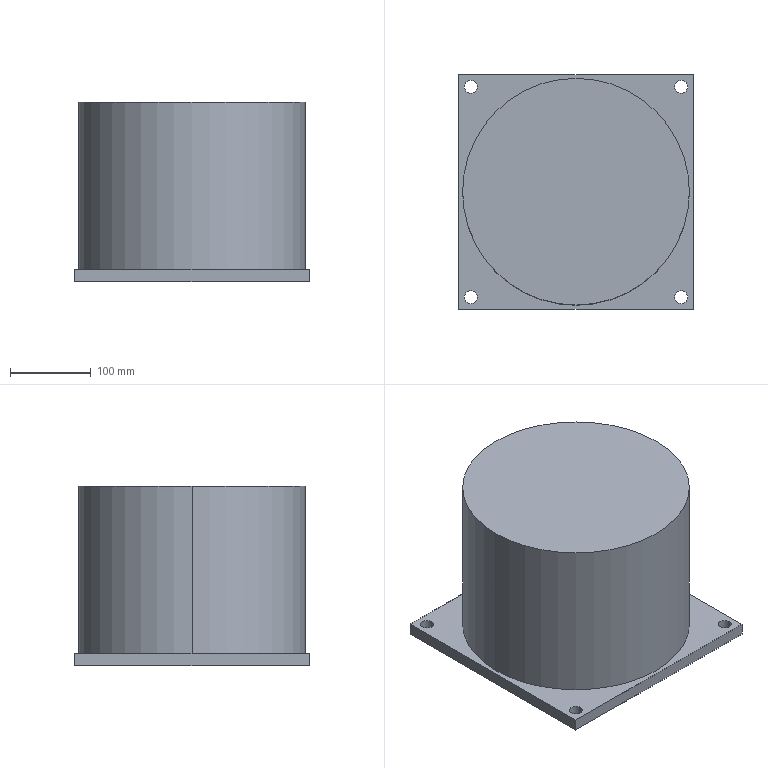Part | NX | 1 solid | 17 faces | box 290 x 290 x 222 mm | volume 13995506 mm3 | cylinder 10 | plane 7 | commonest cylinder face diameters 16 x8 280 x2
STEP:
#1=CARTESIAN_POINT('',(-35.226,-137.015,29.));
#2=VERTEX_POINT('',#1);
#3=CARTESIAN_POINT('',(-315.226,-137.015,29.));
#4=VERTEX_POINT('',#3);
#5=CARTESIAN_POINT('',(-175.226,-137.015,29.));
#6=DIRECTION('',(0.,0.,-1.));
#7=DIRECTION('',(-1.,0.,0.));
#8=AXIS2_PLACEMENT_3D('',#5,#6,#7);
#9=CIRCLE('',#8,140.);
#10=EDGE_CURVE('',#2,#4,#9,.T.);
#11=ORIENTED_EDGE('',*,*,#10,.F.);
#12=CARTESIAN_POINT('',(-35.226,-137.015,236.));
#13=VERTEX_POINT('',#12);
#14=CARTESIAN_POINT('',(-35.226,-137.015,236.));
#15=DIRECTION('',(0.,0.,-1.));
#16=VECTOR('',#15,1000.);
#17=LINE('',#14,#16);
#18=EDGE_CURVE('',#2,#13,#17,.F.);
#19=ORIENTED_EDGE('',*,*,#18,.T.);
#20=CARTESIAN_POINT('',(-315.226,-137.015,236.));
#21=VERTEX_POINT('',#20);
#22=CARTESIAN_POINT('',(-175.226,-137.015,236.));
#23=DIRECTION('',(0.,0.,-1.));
#24=DIRECTION('',(-1.,0.,0.));
#25=AXIS2_PLACEMENT_3D('',#22,#23,#24);
#26=CIRCLE('',#25,140.);
#27=EDGE_CURVE('',#13,#21,#26,.T.);
#28=ORIENTED_EDGE('',*,*,#27,.T.);
#29=CARTESIAN_POINT('',(-315.226,-137.015,236.));
#30=DIRECTION('',(0.,0.,-1.));
#31=VECTOR('',#30,1000.);
#32=LINE('',#29,#31);
#33=EDGE_CURVE('',#4,#21,#32,.F.);
#34=ORIENTED_EDGE('',*,*,#33,.F.);
#35=EDGE_LOOP('',(#11,#19,#28,#34));
#36=FACE_BOUND('',#35,.T.);
#37=CARTESIAN_POINT('',(-175.226,-137.015,236.));
#38=DIRECTION('',(0.,0.,-1.));
#39=DIRECTION('',(-1.,0.,0.));
#40=AXIS2_PLACEMENT_3D('',#37,#38,#39);
#41=CYLINDRICAL_SURFACE('',#40,140.);
#42=ADVANCED_FACE('',(#36),#41,.T.);
#43=CARTESIAN_POINT('',(-320.226,-282.015,29.));
#44=VERTEX_POINT('',#43);
#45=CARTESIAN_POINT('',(-320.226,7.985,29.));
#46=VERTEX_POINT('',#45);
#47=CARTESIAN_POINT('',(-320.226,-137.015,29.));
#48=DIRECTION('',(0.,1.,0.));
#49=VECTOR('',#48,1000.);
#50=LINE('',#47,#49);
#51=EDGE_CURVE('',#44,#46,#50,.T.);
#52=ORIENTED_EDGE('',*,*,#51,.F.);
#53=CARTESIAN_POINT('',(-30.226,-282.015,29.));
#54=VERTEX_POINT('',#53);
#55=CARTESIAN_POINT('',(-175.226,-282.015,29.));
#56=DIRECTION('',(-1.,0.,0.));
#57=VECTOR('',#56,1000.);
#58=LINE('',#55,#57);
#59=EDGE_CURVE('',#54,#44,#58,.T.);
#60=ORIENTED_EDGE('',*,*,#59,.F.);
#61=CARTESIAN_POINT('',(-30.226,7.985,29.));
#62=VERTEX_POINT('',#61);
#63=CARTESIAN_POINT('',(-30.226,-137.015,29.));
#64=DIRECTION('',(0.,1.,0.));
#65=VECTOR('',#64,1000.);
#66=LINE('',#63,#65);
#67=EDGE_CURVE('',#54,#62,#66,.T.);
#68=ORIENTED_EDGE('',*,*,#67,.T.);
#69=CARTESIAN_POINT('',(-175.226,7.985,29.));
#70=DIRECTION('',(-1.,0.,0.));
#71=VECTOR('',#70,1000.);
#72=LINE('',#69,#71);
#73=EDGE_CURVE('',#62,#46,#72,.T.);
#74=ORIENTED_EDGE('',*,*,#73,.T.);
#75=EDGE_LOOP('',(#52,#60,#68,#74));
#76=FACE_BOUND('',#75,.T.);
#77=CARTESIAN_POINT('',(-37.226,-267.015,29.));
#78=VERTEX_POINT('',#77);
#79=CARTESIAN_POINT('',(-53.226,-267.015,29.));
#80=VERTEX_POINT('',#79);
#81=CARTESIAN_POINT('',(-45.226,-267.015,29.));
#82=DIRECTION('',(0.,0.,-1.));
#83=DIRECTION('',(-1.,0.,0.));
#84=AXIS2_PLACEMENT_3D('',#81,#82,#83);
#85=CIRCLE('',#84,8.);
#86=EDGE_CURVE('',#78,#80,#85,.T.);
#87=ORIENTED_EDGE('',*,*,#86,.T.);
#88=CARTESIAN_POINT('',(-45.226,-267.015,29.));
#89=DIRECTION('',(0.,0.,-1.));
#90=DIRECTION('',(-1.,0.,0.));
#91=AXIS2_PLACEMENT_3D('',#88,#89,#90);
#92=CIRCLE('',#91,8.);
#93=EDGE_CURVE('',#80,#78,#92,.T.);
#94=ORIENTED_EDGE('',*,*,#93,.T.);
#95=EDGE_LOOP('',(#87,#94));
#96=FACE_BOUND('',#95,.T.);
#97=CARTESIAN_POINT('',(-297.226,-267.015,29.));
#98=VERTEX_POINT('',#97);
#99=CARTESIAN_POINT('',(-313.226,-267.015,29.));
#100=VERTEX_POINT('',#99);
#101=CARTESIAN_POINT('',(-305.226,-267.015,29.));
#102=DIRECTION('',(0.,0.,-1.));
#103=DIRECTION('',(-1.,0.,0.));
#104=AXIS2_PLACEMENT_3D('',#101,#102,#103);
#105=CIRCLE('',#104,8.);
#106=EDGE_CURVE('',#98,#100,#105,.T.);
#107=ORIENTED_EDGE('',*,*,#106,.T.);
#108=CARTESIAN_POINT('',(-305.226,-267.015,29.));
#109=DIRECTION('',(0.,0.,-1.));
#110=DIRECTION('',(-1.,0.,0.));
#111=AXIS2_PLACEMENT_3D('',#108,#109,#110);
#112=CIRCLE('',#111,8.);
#113=EDGE_CURVE('',#100,#98,#112,.T.);
#114=ORIENTED_EDGE('',*,*,#113,.T.);
#115=EDGE_LOOP('',(#107,#114));
#116=FACE_BOUND('',#115,.T.);
#117=CARTESIAN_POINT('',(-37.226,-7.015,29.));
#118=VERTEX_POINT('',#117);
#119=CARTESIAN_POINT('',(-53.226,-7.015,29.));
#120=VERTEX_POINT('',#119);
#121=CARTESIAN_POINT('',(-45.226,-7.015,29.));
#122=DIRECTION('',(0.,0.,-1.));
#123=DIRECTION('',(-1.,0.,0.));
#124=AXIS2_PLACEMENT_3D('',#121,#122,#123);
#125=CIRCLE('',#124,8.);
#126=EDGE_CURVE('',#118,#120,#125,.T.);
#127=ORIENTED_EDGE('',*,*,#126,.T.);
#128=CARTESIAN_POINT('',(-45.226,-7.015,29.));
#129=DIRECTION('',(0.,0.,-1.));
#130=DIRECTION('',(-1.,0.,0.));
#131=AXIS2_PLACEMENT_3D('',#128,#129,#130);
#132=CIRCLE('',#131,8.);
#133=EDGE_CURVE('',#120,#118,#132,.T.);
#134=ORIENTED_EDGE('',*,*,#133,.T.);
#135=EDGE_LOOP('',(#127,#134));
#136=FACE_BOUND('',#135,.T.);
#137=CARTESIAN_POINT('',(-297.226,-7.015,29.));
#138=VERTEX_POINT('',#137);
#139=CARTESIAN_POINT('',(-313.226,-7.015,29.));
#140=VERTEX_POINT('',#139);
#141=CARTESIAN_POINT('',(-305.226,-7.015,29.));
#142=DIRECTION('',(0.,0.,-1.));
#143=DIRECTION('',(-1.,0.,0.));
#144=AXIS2_PLACEMENT_3D('',#141,#142,#143);
#145=CIRCLE('',#144,8.);
#146=EDGE_CURVE('',#138,#140,#145,.T.);
#147=ORIENTED_EDGE('',*,*,#146,.T.);
#148=CARTESIAN_POINT('',(-305.226,-7.015,29.));
#149=DIRECTION('',(0.,0.,-1.));
#150=DIRECTION('',(-1.,0.,0.));
#151=AXIS2_PLACEMENT_3D('',#148,#149,#150);
#152=CIRCLE('',#151,8.);
#153=EDGE_CURVE('',#140,#138,#152,.T.);
#154=ORIENTED_EDGE('',*,*,#153,.T.);
#155=EDGE_LOOP('',(#147,#154));
#156=FACE_BOUND('',#155,.T.);
#157=ORIENTED_EDGE('',*,*,#10,.T.);
#158=CARTESIAN_POINT('',(-175.226,-137.015,29.));
#159=DIRECTION('',(0.,0.,-1.));
#160=DIRECTION('',(-1.,0.,0.));
#161=AXIS2_PLACEMENT_3D('',#158,#159,#160);
#162=CIRCLE('',#161,140.);
#163=EDGE_CURVE('',#4,#2,#162,.T.);
#164=ORIENTED_EDGE('',*,*,#163,.T.);
#165=EDGE_LOOP('',(#157,#164));
#166=FACE_BOUND('',#165,.T.);
#167=CARTESIAN_POINT('',(-181.149,-97.75,29.));
#168=DIRECTION('',(0.,0.,-1.));
#169=DIRECTION('',(0.,-1.,0.));
#170=AXIS2_PLACEMENT_3D('',#167,#168,#169);
#171=PLANE('',#170);
#172=ADVANCED_FACE('',(#76,#96,#116,#136,#156,#166),#171,.F.);
#173=ORIENTED_EDGE('',*,*,#73,.F.);
#174=CARTESIAN_POINT('',(-30.226,7.985,14.));
#175=VERTEX_POINT('',#174);
#176=CARTESIAN_POINT('',(-30.226,7.985,29.));
#177=DIRECTION('',(0.,0.,-1.));
#178=VECTOR('',#177,1000.);
#179=LINE('',#176,#178);
#180=EDGE_CURVE('',#62,#175,#179,.T.);
#181=ORIENTED_EDGE('',*,*,#180,.T.);
#182=CARTESIAN_POINT('',(-320.226,7.985,14.));
#183=VERTEX_POINT('',#182);
#184=CARTESIAN_POINT('',(-175.226,7.985,14.));
#185=DIRECTION('',(-1.,0.,0.));
#186=VECTOR('',#185,1000.);
#187=LINE('',#184,#186);
#188=EDGE_CURVE('',#175,#183,#187,.T.);
#189=ORIENTED_EDGE('',*,*,#188,.T.);
#190=CARTESIAN_POINT('',(-320.226,7.985,29.));
#191=DIRECTION('',(0.,0.,-1.));
#192=VECTOR('',#191,1000.);
#193=LINE('',#190,#192);
#194=EDGE_CURVE('',#46,#183,#193,.T.);
#195=ORIENTED_EDGE('',*,*,#194,.F.);
#196=EDGE_LOOP('',(#173,#181,#189,#195));
#197=FACE_BOUND('',#196,.T.);
#198=CARTESIAN_POINT('',(-30.226,7.985,29.));
#199=DIRECTION('',(0.,1.,0.));
#200=DIRECTION('',(1.,0.,0.));
#201=AXIS2_PLACEMENT_3D('',#198,#199,#200);
#202=PLANE('',#201);
#203=ADVANCED_FACE('',(#197),#202,.T.);
#204=ORIENTED_EDGE('',*,*,#59,.T.);
#205=CARTESIAN_POINT('',(-320.226,-282.015,14.));
#206=VERTEX_POINT('',#205);
#207=CARTESIAN_POINT('',(-320.226,-282.015,29.));
#208=DIRECTION('',(0.,0.,-1.));
#209=VECTOR('',#208,1000.);
#210=LINE('',#207,#209);
#211=EDGE_CURVE('',#44,#206,#210,.T.);
#212=ORIENTED_EDGE('',*,*,#211,.T.);
#213=CARTESIAN_POINT('',(-30.226,-282.015,14.));
#214=VERTEX_POINT('',#213);
#215=CARTESIAN_POINT('',(-175.226,-282.015,14.));
#216=DIRECTION('',(-1.,0.,0.));
#217=VECTOR('',#216,1000.);
#218=LINE('',#215,#217);
#219=EDGE_CURVE('',#214,#206,#218,.T.);
#220=ORIENTED_EDGE('',*,*,#219,.F.);
#221=CARTESIAN_POINT('',(-30.226,-282.015,29.));
#222=DIRECTION('',(0.,0.,-1.));
#223=VECTOR('',#222,1000.);
#224=LINE('',#221,#223);
#225=EDGE_CURVE('',#54,#214,#224,.T.);
#226=ORIENTED_EDGE('',*,*,#225,.F.);
#227=EDGE_LOOP('',(#204,#212,#220,#226));
#228=FACE_BOUND('',#227,.T.);
#229=CARTESIAN_POINT('',(-320.226,-282.015,29.));
#230=DIRECTION('',(0.,-1.,0.));
#231=DIRECTION('',(0.,0.,-1.));
#232=AXIS2_PLACEMENT_3D('',#229,#230,#231);
#233=PLANE('',#232);
#234=ADVANCED_FACE('',(#228),#233,.T.);
#235=ORIENTED_EDGE('',*,*,#67,.F.);
#236=ORIENTED_EDGE('',*,*,#225,.T.);
#237=CARTESIAN_POINT('',(-30.226,-137.015,14.));
#238=DIRECTION('',(0.,1.,0.));
#239=VECTOR('',#238,1000.);
#240=LINE('',#237,#239);
#241=EDGE_CURVE('',#214,#175,#240,.T.);
#242=ORIENTED_EDGE('',*,*,#241,.T.);
#243=ORIENTED_EDGE('',*,*,#180,.F.);
#244=EDGE_LOOP('',(#235,#236,#242,#243));
#245=FACE_BOUND('',#244,.T.);
#246=CARTESIAN_POINT('',(-30.226,-282.015,29.));
#247=DIRECTION('',(1.,0.,0.));
#248=DIRECTION('',(0.,1.,0.));
#249=AXIS2_PLACEMENT_3D('',#246,#247,#248);
#250=PLANE('',#249);
#251=ADVANCED_FACE('',(#245),#250,.T.);
#252=ORIENTED_EDGE('',*,*,#51,.T.);
#253=ORIENTED_EDGE('',*,*,#194,.T.);
#254=CARTESIAN_POINT('',(-320.226,-137.015,14.));
#255=DIRECTION('',(0.,1.,0.));
#256=VECTOR('',#255,1000.);
#257=LINE('',#254,#256);
#258=EDGE_CURVE('',#206,#183,#257,.T.);
#259=ORIENTED_EDGE('',*,*,#258,.F.);
#260=ORIENTED_EDGE('',*,*,#211,.F.);
#261=EDGE_LOOP('',(#252,#253,#259,#260));
#262=FACE_BOUND('',#261,.T.);
#263=CARTESIAN_POINT('',(-320.226,7.985,29.));
#264=DIRECTION('',(-1.,0.,0.));
#265=DIRECTION('',(0.,0.,1.));
#266=AXIS2_PLACEMENT_3D('',#263,#264,#265);
#267=PLANE('',#266);
#268=ADVANCED_FACE('',(#262),#267,.T.);
#269=ORIENTED_EDGE('',*,*,#188,.F.);
#270=ORIENTED_EDGE('',*,*,#241,.F.);
#271=ORIENTED_EDGE('',*,*,#219,.T.);
#272=ORIENTED_EDGE('',*,*,#258,.T.);
#273=EDGE_LOOP('',(#269,#270,#271,#272));
#274=FACE_BOUND('',#273,.T.);
#275=CARTESIAN_POINT('',(-37.226,-267.015,14.));
#276=VERTEX_POINT('',#275);
#277=CARTESIAN_POINT('',(-53.226,-267.015,14.));
#278=VERTEX_POINT('',#277);
#279=CARTESIAN_POINT('',(-45.226,-267.015,14.));
#280=DIRECTION('',(0.,0.,-1.));
#281=DIRECTION('',(-1.,0.,0.));
#282=AXIS2_PLACEMENT_3D('',#279,#280,#281);
#283=CIRCLE('',#282,8.);
#284=EDGE_CURVE('',#276,#278,#283,.T.);
#285=ORIENTED_EDGE('',*,*,#284,.F.);
#286=CARTESIAN_POINT('',(-45.226,-267.015,14.));
#287=DIRECTION('',(0.,0.,-1.));
#288=DIRECTION('',(-1.,0.,0.));
#289=AXIS2_PLACEMENT_3D('',#286,#287,#288);
#290=CIRCLE('',#289,8.);
#291=EDGE_CURVE('',#278,#276,#290,.T.);
#292=ORIENTED_EDGE('',*,*,#291,.F.);
#293=EDGE_LOOP('',(#285,#292));
#294=FACE_BOUND('',#293,.T.);
#295=CARTESIAN_POINT('',(-297.226,-267.015,14.));
#296=VERTEX_POINT('',#295);
#297=CARTESIAN_POINT('',(-313.226,-267.015,14.));
#298=VERTEX_POINT('',#297);
#299=CARTESIAN_POINT('',(-305.226,-267.015,14.));
#300=DIRECTION('',(0.,0.,-1.));
#301=DIRECTION('',(-1.,0.,0.));
#302=AXIS2_PLACEMENT_3D('',#299,#300,#301);
#303=CIRCLE('',#302,8.);
#304=EDGE_CURVE('',#296,#298,#303,.T.);
#305=ORIENTED_EDGE('',*,*,#304,.F.);
#306=CARTESIAN_POINT('',(-305.226,-267.015,14.));
#307=DIRECTION('',(0.,0.,-1.));
#308=DIRECTION('',(-1.,0.,0.));
#309=AXIS2_PLACEMENT_3D('',#306,#307,#308);
#310=CIRCLE('',#309,8.);
#311=EDGE_CURVE('',#298,#296,#310,.T.);
#312=ORIENTED_EDGE('',*,*,#311,.F.);
#313=EDGE_LOOP('',(#305,#312));
#314=FACE_BOUND('',#313,.T.);
#315=CARTESIAN_POINT('',(-37.226,-7.015,14.));
#316=VERTEX_POINT('',#315);
#317=CARTESIAN_POINT('',(-53.226,-7.015,14.));
#318=VERTEX_POINT('',#317);
#319=CARTESIAN_POINT('',(-45.226,-7.015,14.));
#320=DIRECTION('',(0.,0.,-1.));
#321=DIRECTION('',(-1.,0.,0.));
#322=AXIS2_PLACEMENT_3D('',#319,#320,#321);
#323=CIRCLE('',#322,8.);
#324=EDGE_CURVE('',#316,#318,#323,.T.);
#325=ORIENTED_EDGE('',*,*,#324,.F.);
#326=CARTESIAN_POINT('',(-45.226,-7.015,14.));
#327=DIRECTION('',(0.,0.,-1.));
#328=DIRECTION('',(-1.,0.,0.));
#329=AXIS2_PLACEMENT_3D('',#326,#327,#328);
#330=CIRCLE('',#329,8.);
#331=EDGE_CURVE('',#318,#316,#330,.T.);
#332=ORIENTED_EDGE('',*,*,#331,.F.);
#333=EDGE_LOOP('',(#325,#332));
#334=FACE_BOUND('',#333,.T.);
#335=CARTESIAN_POINT('',(-297.226,-7.015,14.));
#336=VERTEX_POINT('',#335);
#337=CARTESIAN_POINT('',(-313.226,-7.015,14.));
#338=VERTEX_POINT('',#337);
#339=CARTESIAN_POINT('',(-305.226,-7.015,14.));
#340=DIRECTION('',(0.,0.,-1.));
#341=DIRECTION('',(-1.,0.,0.));
#342=AXIS2_PLACEMENT_3D('',#339,#340,#341);
#343=CIRCLE('',#342,8.);
#344=EDGE_CURVE('',#336,#338,#343,.T.);
#345=ORIENTED_EDGE('',*,*,#344,.F.);
#346=CARTESIAN_POINT('',(-305.226,-7.015,14.));
#347=DIRECTION('',(0.,0.,-1.));
#348=DIRECTION('',(-1.,0.,0.));
#349=AXIS2_PLACEMENT_3D('',#346,#347,#348);
#350=CIRCLE('',#349,8.);
#351=EDGE_CURVE('',#338,#336,#350,.T.);
#352=ORIENTED_EDGE('',*,*,#351,.F.);
#353=EDGE_LOOP('',(#345,#352));
#354=FACE_BOUND('',#353,.T.);
#355=CARTESIAN_POINT('',(-181.149,-97.75,14.));
#356=DIRECTION('',(0.,0.,-1.));
#357=DIRECTION('',(0.,-1.,0.));
#358=AXIS2_PLACEMENT_3D('',#355,#356,#357);
#359=PLANE('',#358);
#360=ADVANCED_FACE('',(#274,#294,#314,#334,#354),#359,.T.);
#361=ORIENTED_EDGE('',*,*,#284,.T.);
#362=CARTESIAN_POINT('',(-53.226,-267.015,29.));
#363=DIRECTION('',(0.,0.,-1.));
#364=VECTOR('',#363,1000.);
#365=LINE('',#362,#364);
#366=EDGE_CURVE('',#278,#80,#365,.F.);
#367=ORIENTED_EDGE('',*,*,#366,.T.);
#368=ORIENTED_EDGE('',*,*,#86,.F.);
#369=CARTESIAN_POINT('',(-37.226,-267.015,29.));
#370=DIRECTION('',(0.,0.,-1.));
#371=VECTOR('',#370,1000.);
#372=LINE('',#369,#371);
#373=EDGE_CURVE('',#276,#78,#372,.F.);
#374=ORIENTED_EDGE('',*,*,#373,.F.);
#375=EDGE_LOOP('',(#361,#367,#368,#374));
#376=FACE_BOUND('',#375,.T.);
#377=CARTESIAN_POINT('',(-45.226,-267.015,29.));
#378=DIRECTION('',(0.,0.,-1.));
#379=DIRECTION('',(-1.,0.,0.));
#380=AXIS2_PLACEMENT_3D('',#377,#378,#379);
#381=CYLINDRICAL_SURFACE('',#380,8.);
#382=ADVANCED_FACE('',(#376),#381,.F.);
#383=ORIENTED_EDGE('',*,*,#304,.T.);
#384=CARTESIAN_POINT('',(-313.226,-267.015,29.));
#385=DIRECTION('',(0.,0.,-1.));
#386=VECTOR('',#385,1000.);
#387=LINE('',#384,#386);
#388=EDGE_CURVE('',#298,#100,#387,.F.);
#389=ORIENTED_EDGE('',*,*,#388,.T.);
#390=ORIENTED_EDGE('',*,*,#106,.F.);
#391=CARTESIAN_POINT('',(-297.226,-267.015,29.));
#392=DIRECTION('',(0.,0.,-1.));
#393=VECTOR('',#392,1000.);
#394=LINE('',#391,#393);
#395=EDGE_CURVE('',#296,#98,#394,.F.);
#396=ORIENTED_EDGE('',*,*,#395,.F.);
#397=EDGE_LOOP('',(#383,#389,#390,#396));
#398=FACE_BOUND('',#397,.T.);
#399=CARTESIAN_POINT('',(-305.226,-267.015,29.));
#400=DIRECTION('',(0.,0.,-1.));
#401=DIRECTION('',(-1.,0.,0.));
#402=AXIS2_PLACEMENT_3D('',#399,#400,#401);
#403=CYLINDRICAL_SURFACE('',#402,8.);
#404=ADVANCED_FACE('',(#398),#403,.F.);
#405=ORIENTED_EDGE('',*,*,#324,.T.);
#406=CARTESIAN_POINT('',(-53.226,-7.015,29.));
#407=DIRECTION('',(0.,0.,-1.));
#408=VECTOR('',#407,1000.);
#409=LINE('',#406,#408);
#410=EDGE_CURVE('',#318,#120,#409,.F.);
#411=ORIENTED_EDGE('',*,*,#410,.T.);
#412=ORIENTED_EDGE('',*,*,#126,.F.);
#413=CARTESIAN_POINT('',(-37.226,-7.015,29.));
#414=DIRECTION('',(0.,0.,-1.));
#415=VECTOR('',#414,1000.);
#416=LINE('',#413,#415);
#417=EDGE_CURVE('',#316,#118,#416,.F.);
#418=ORIENTED_EDGE('',*,*,#417,.F.);
#419=EDGE_LOOP('',(#405,#411,#412,#418));
#420=FACE_BOUND('',#419,.T.);
#421=CARTESIAN_POINT('',(-45.226,-7.015,29.));
#422=DIRECTION('',(0.,0.,-1.));
#423=DIRECTION('',(-1.,0.,0.));
#424=AXIS2_PLACEMENT_3D('',#421,#422,#423);
#425=CYLINDRICAL_SURFACE('',#424,8.);
#426=ADVANCED_FACE('',(#420),#425,.F.);
#427=ORIENTED_EDGE('',*,*,#344,.T.);
#428=CARTESIAN_POINT('',(-313.226,-7.015,29.));
#429=DIRECTION('',(0.,0.,-1.));
#430=VECTOR('',#429,1000.);
#431=LINE('',#428,#430);
#432=EDGE_CURVE('',#338,#140,#431,.F.);
#433=ORIENTED_EDGE('',*,*,#432,.T.);
#434=ORIENTED_EDGE('',*,*,#146,.F.);
#435=CARTESIAN_POINT('',(-297.226,-7.015,29.));
#436=DIRECTION('',(0.,0.,-1.));
#437=VECTOR('',#436,1000.);
#438=LINE('',#435,#437);
#439=EDGE_CURVE('',#336,#138,#438,.F.);
#440=ORIENTED_EDGE('',*,*,#439,.F.);
#441=EDGE_LOOP('',(#427,#433,#434,#440));
#442=FACE_BOUND('',#441,.T.);
#443=CARTESIAN_POINT('',(-305.226,-7.015,29.));
#444=DIRECTION('',(0.,0.,-1.));
#445=DIRECTION('',(-1.,0.,0.));
#446=AXIS2_PLACEMENT_3D('',#443,#444,#445);
#447=CYLINDRICAL_SURFACE('',#446,8.);
#448=ADVANCED_FACE('',(#442),#447,.F.);
#449=ORIENTED_EDGE('',*,*,#432,.F.);
#450=ORIENTED_EDGE('',*,*,#351,.T.);
#451=ORIENTED_EDGE('',*,*,#439,.T.);
#452=ORIENTED_EDGE('',*,*,#153,.F.);
#453=EDGE_LOOP('',(#449,#450,#451,#452));
#454=FACE_BOUND('',#453,.T.);
#455=CARTESIAN_POINT('',(-305.226,-7.015,29.));
#456=DIRECTION('',(0.,0.,-1.));
#457=DIRECTION('',(-1.,0.,0.));
#458=AXIS2_PLACEMENT_3D('',#455,#456,#457);
#459=CYLINDRICAL_SURFACE('',#458,8.);
#460=ADVANCED_FACE('',(#454),#459,.F.);
#461=ORIENTED_EDGE('',*,*,#410,.F.);
#462=ORIENTED_EDGE('',*,*,#331,.T.);
#463=ORIENTED_EDGE('',*,*,#417,.T.);
#464=ORIENTED_EDGE('',*,*,#133,.F.);
#465=EDGE_LOOP('',(#461,#462,#463,#464));
#466=FACE_BOUND('',#465,.T.);
#467=CARTESIAN_POINT('',(-45.226,-7.015,29.));
#468=DIRECTION('',(0.,0.,-1.));
#469=DIRECTION('',(-1.,0.,0.));
#470=AXIS2_PLACEMENT_3D('',#467,#468,#469);
#471=CYLINDRICAL_SURFACE('',#470,8.);
#472=ADVANCED_FACE('',(#466),#471,.F.);
#473=ORIENTED_EDGE('',*,*,#388,.F.);
#474=ORIENTED_EDGE('',*,*,#311,.T.);
#475=ORIENTED_EDGE('',*,*,#395,.T.);
#476=ORIENTED_EDGE('',*,*,#113,.F.);
#477=EDGE_LOOP('',(#473,#474,#475,#476));
#478=FACE_BOUND('',#477,.T.);
#479=CARTESIAN_POINT('',(-305.226,-267.015,29.));
#480=DIRECTION('',(0.,0.,-1.));
#481=DIRECTION('',(-1.,0.,0.));
#482=AXIS2_PLACEMENT_3D('',#479,#480,#481);
#483=CYLINDRICAL_SURFACE('',#482,8.);
#484=ADVANCED_FACE('',(#478),#483,.F.);
#485=ORIENTED_EDGE('',*,*,#33,.T.);
#486=CARTESIAN_POINT('',(-175.226,-137.015,236.));
#487=DIRECTION('',(0.,0.,-1.));
#488=DIRECTION('',(-1.,0.,0.));
#489=AXIS2_PLACEMENT_3D('',#486,#487,#488);
#490=CIRCLE('',#489,140.);
#491=EDGE_CURVE('',#21,#13,#490,.T.);
#492=ORIENTED_EDGE('',*,*,#491,.T.);
#493=ORIENTED_EDGE('',*,*,#18,.F.);
#494=ORIENTED_EDGE('',*,*,#163,.F.);
#495=EDGE_LOOP('',(#485,#492,#493,#494));
#496=FACE_BOUND('',#495,.T.);
#497=CARTESIAN_POINT('',(-175.226,-137.015,236.));
#498=DIRECTION('',(0.,0.,-1.));
#499=DIRECTION('',(-1.,0.,0.));
#500=AXIS2_PLACEMENT_3D('',#497,#498,#499);
#501=CYLINDRICAL_SURFACE('',#500,140.);
#502=ADVANCED_FACE('',(#496),#501,.T.);
#503=ORIENTED_EDGE('',*,*,#366,.F.);
#504=ORIENTED_EDGE('',*,*,#291,.T.);
#505=ORIENTED_EDGE('',*,*,#373,.T.);
#506=ORIENTED_EDGE('',*,*,#93,.F.);
#507=EDGE_LOOP('',(#503,#504,#505,#506));
#508=FACE_BOUND('',#507,.T.);
#509=CARTESIAN_POINT('',(-45.226,-267.015,29.));
#510=DIRECTION('',(0.,0.,-1.));
#511=DIRECTION('',(-1.,0.,0.));
#512=AXIS2_PLACEMENT_3D('',#509,#510,#511);
#513=CYLINDRICAL_SURFACE('',#512,8.);
#514=ADVANCED_FACE('',(#508),#513,.F.);
#515=ORIENTED_EDGE('',*,*,#27,.F.);
#516=ORIENTED_EDGE('',*,*,#491,.F.);
#517=EDGE_LOOP('',(#515,#516));
#518=FACE_BOUND('',#517,.T.);
#519=CARTESIAN_POINT('',(-106.56,-178.326,236.));
#520=DIRECTION('',(0.,0.,-1.));
#521=DIRECTION('',(0.,-1.,0.));
#522=AXIS2_PLACEMENT_3D('',#519,#520,#521);
#523=PLANE('',#522);
#524=ADVANCED_FACE('',(#518),#523,.F.);
#525=CLOSED_SHELL('',(#42,#172,#203,#234,#251,#268,#360,#382,#404,#426,#448,#460,#472,#484,#502,#514,#524));
#526=MANIFOLD_SOLID_BREP('',#525);
#527=(LENGTH_UNIT()NAMED_UNIT(*)SI_UNIT(.MILLI.,.METRE.));
#528=UNCERTAINTY_MEASURE_WITH_UNIT(LENGTH_MEASURE(0.00001),#527,'','');
#529=(NAMED_UNIT(*)PLANE_ANGLE_UNIT()SI_UNIT($,.RADIAN.));
#530=(NAMED_UNIT(*)SI_UNIT($,.STERADIAN.)SOLID_ANGLE_UNIT());
#531=(GEOMETRIC_REPRESENTATION_CONTEXT(3)GLOBAL_UNCERTAINTY_ASSIGNED_CONTEXT((#528))GLOBAL_UNIT_ASSIGNED_CONTEXT((#527,#529,#530))REPRESENTATION_CONTEXT('',''));
#532=ADVANCED_BREP_SHAPE_REPRESENTATION('',(#526),#531);